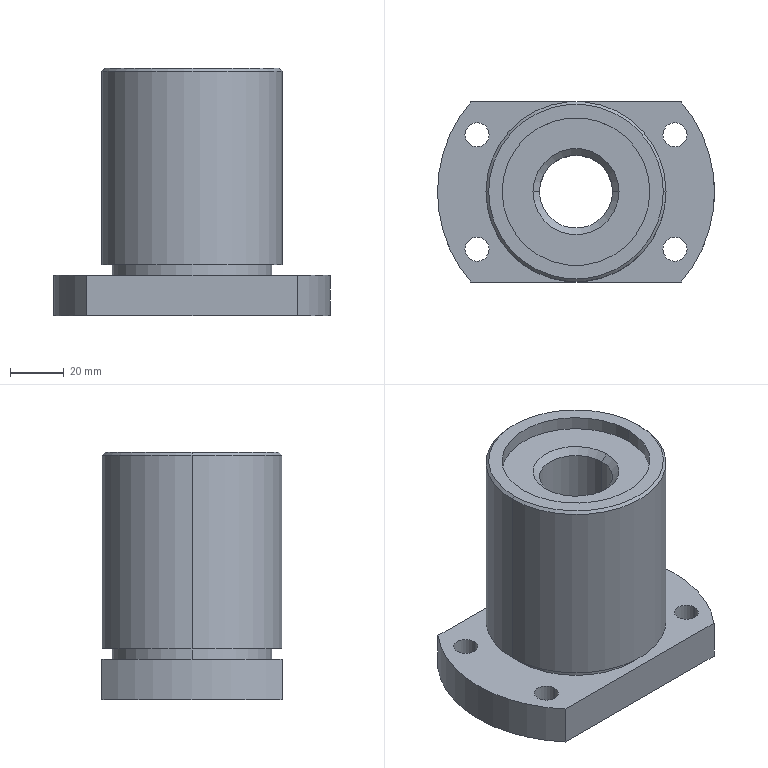Part | SolidWorks | features BaseBody 1 | 1 solid | 39 faces | box 103 x 67 x 92 mm | volume 287626 mm3 | cylinder 23 | cone 8 | plane 8 | commonest cylinder face diameters 9 x8 55 x4 103 x3 4.917 x2 27.2 x2 59.3 x2
STEP:
#1=CARTESIAN_POINT('',(211.71,1592.079,-1039.15));
#2=VERTEX_POINT('',#1);
#3=CARTESIAN_POINT('',(144.71,1592.079,-1039.15));
#4=VERTEX_POINT('',#3);
#5=CARTESIAN_POINT('',(178.21,1592.079,-1039.15));
#6=DIRECTION('',(0.,0.,1.));
#7=DIRECTION('',(1.,0.,0.));
#8=AXIS2_PLACEMENT_3D('',#5,#6,#7);
#9=CIRCLE('',#8,33.5);
#10=EDGE_CURVE('',#2,#4,#9,.T.);
#11=ORIENTED_EDGE('',*,*,#10,.T.);
#12=CARTESIAN_POINT('',(144.71,1592.079,-967.));
#13=VERTEX_POINT('',#12);
#14=CARTESIAN_POINT('',(144.71,1592.079,-1043.));
#15=DIRECTION('',(0.,0.,1.));
#16=VECTOR('',#15,1000.);
#17=LINE('',#14,#16);
#18=EDGE_CURVE('',#4,#13,#17,.T.);
#19=ORIENTED_EDGE('',*,*,#18,.T.);
#20=CARTESIAN_POINT('',(211.71,1592.079,-967.));
#21=VERTEX_POINT('',#20);
#22=CARTESIAN_POINT('',(178.21,1592.079,-967.));
#23=DIRECTION('',(0.,0.,-1.));
#24=DIRECTION('',(1.,0.,0.));
#25=AXIS2_PLACEMENT_3D('',#22,#23,#24);
#26=CIRCLE('',#25,33.5);
#27=EDGE_CURVE('',#13,#21,#26,.T.);
#28=ORIENTED_EDGE('',*,*,#27,.T.);
#29=CARTESIAN_POINT('',(211.71,1592.079,-1043.));
#30=DIRECTION('',(0.,0.,1.));
#31=VECTOR('',#30,1000.);
#32=LINE('',#29,#31);
#33=EDGE_CURVE('',#2,#21,#32,.T.);
#34=ORIENTED_EDGE('',*,*,#33,.F.);
#35=EDGE_LOOP('',(#11,#19,#28,#34));
#36=FACE_OUTER_BOUND('',#35,.T.);
#37=CARTESIAN_POINT('',(178.21,1592.079,-1043.));
#38=DIRECTION('',(0.,0.,1.));
#39=DIRECTION('',(1.,0.,0.));
#40=AXIS2_PLACEMENT_3D('',#37,#38,#39);
#41=CYLINDRICAL_SURFACE('',#40,33.5);
#42=ADVANCED_FACE('',(#36),#41,.T.);
#43=CARTESIAN_POINT('',(145.71,1592.079,-966.));
#44=VERTEX_POINT('',#43);
#45=CARTESIAN_POINT('',(210.71,1592.079,-966.));
#46=VERTEX_POINT('',#45);
#47=CARTESIAN_POINT('',(178.21,1592.079,-966.));
#48=DIRECTION('',(0.,0.,-1.));
#49=DIRECTION('',(-1.,0.,0.));
#50=AXIS2_PLACEMENT_3D('',#47,#48,#49);
#51=CIRCLE('',#50,32.5);
#52=EDGE_CURVE('',#44,#46,#51,.T.);
#53=ORIENTED_EDGE('',*,*,#52,.T.);
#54=CARTESIAN_POINT('',(211.71,1592.079,-967.));
#55=DIRECTION('',(0.7071,0.,-0.7071));
#56=VECTOR('',#55,1000.);
#57=LINE('',#54,#56);
#58=EDGE_CURVE('',#46,#21,#57,.T.);
#59=ORIENTED_EDGE('',*,*,#58,.T.);
#60=ORIENTED_EDGE('',*,*,#27,.F.);
#61=CARTESIAN_POINT('',(144.71,1592.079,-967.));
#62=DIRECTION('',(-0.7071,0.,-0.7071));
#63=VECTOR('',#62,1000.);
#64=LINE('',#61,#63);
#65=EDGE_CURVE('',#44,#13,#64,.T.);
#66=ORIENTED_EDGE('',*,*,#65,.F.);
#67=EDGE_LOOP('',(#53,#59,#60,#66));
#68=FACE_OUTER_BOUND('',#67,.T.);
#69=CARTESIAN_POINT('',(178.21,1592.079,-967.));
#70=DIRECTION('',(0.,0.,-1.));
#71=DIRECTION('',(-1.,0.,0.));
#72=AXIS2_PLACEMENT_3D('',#69,#70,#71);
#73=CONICAL_SURFACE('',#72,33.5,0.7854);
#74=ADVANCED_FACE('',(#68),#73,.T.);
#75=CARTESIAN_POINT('',(207.86,1592.079,-1043.));
#76=VERTEX_POINT('',#75);
#77=CARTESIAN_POINT('',(148.56,1592.079,-1043.));
#78=VERTEX_POINT('',#77);
#79=CARTESIAN_POINT('',(178.21,1592.079,-1043.));
#80=DIRECTION('',(0.,0.,1.));
#81=DIRECTION('',(1.,0.,0.));
#82=AXIS2_PLACEMENT_3D('',#79,#80,#81);
#83=CIRCLE('',#82,29.65);
#84=EDGE_CURVE('',#76,#78,#83,.T.);
#85=ORIENTED_EDGE('',*,*,#84,.T.);
#86=CARTESIAN_POINT('',(148.56,1592.079,-1039.15));
#87=VERTEX_POINT('',#86);
#88=CARTESIAN_POINT('',(148.56,1592.079,-1043.));
#89=DIRECTION('',(0.,0.,1.));
#90=VECTOR('',#89,1000.);
#91=LINE('',#88,#90);
#92=EDGE_CURVE('',#78,#87,#91,.T.);
#93=ORIENTED_EDGE('',*,*,#92,.T.);
#94=CARTESIAN_POINT('',(207.86,1592.079,-1039.15));
#95=VERTEX_POINT('',#94);
#96=CARTESIAN_POINT('',(178.21,1592.079,-1039.15));
#97=DIRECTION('',(0.,0.,-1.));
#98=DIRECTION('',(1.,0.,0.));
#99=AXIS2_PLACEMENT_3D('',#96,#97,#98);
#100=CIRCLE('',#99,29.65);
#101=EDGE_CURVE('',#87,#95,#100,.T.);
#102=ORIENTED_EDGE('',*,*,#101,.T.);
#103=CARTESIAN_POINT('',(207.86,1592.079,-1043.));
#104=DIRECTION('',(0.,0.,1.));
#105=VECTOR('',#104,1000.);
#106=LINE('',#103,#105);
#107=EDGE_CURVE('',#76,#95,#106,.T.);
#108=ORIENTED_EDGE('',*,*,#107,.F.);
#109=EDGE_LOOP('',(#85,#93,#102,#108));
#110=FACE_OUTER_BOUND('',#109,.T.);
#111=CARTESIAN_POINT('',(178.21,1592.079,-1043.));
#112=DIRECTION('',(0.,0.,1.));
#113=DIRECTION('',(1.,0.,0.));
#114=AXIS2_PLACEMENT_3D('',#111,#112,#113);
#115=CYLINDRICAL_SURFACE('',#114,29.65);
#116=ADVANCED_FACE('',(#110),#115,.T.);
#117=CARTESIAN_POINT('',(150.71,1592.079,-971.));
#118=VERTEX_POINT('',#117);
#119=CARTESIAN_POINT('',(205.71,1592.079,-971.));
#120=VERTEX_POINT('',#119);
#121=CARTESIAN_POINT('',(178.21,1592.079,-971.));
#122=DIRECTION('',(0.,0.,1.));
#123=DIRECTION('',(1.,0.,0.));
#124=AXIS2_PLACEMENT_3D('',#121,#122,#123);
#125=CIRCLE('',#124,27.5);
#126=EDGE_CURVE('',#118,#120,#125,.T.);
#127=ORIENTED_EDGE('',*,*,#126,.F.);
#128=CARTESIAN_POINT('',(150.71,1592.079,-966.));
#129=VERTEX_POINT('',#128);
#130=CARTESIAN_POINT('',(150.71,1592.079,-1043.));
#131=DIRECTION('',(0.,0.,1.));
#132=VECTOR('',#131,1000.);
#133=LINE('',#130,#132);
#134=EDGE_CURVE('',#118,#129,#133,.T.);
#135=ORIENTED_EDGE('',*,*,#134,.T.);
#136=CARTESIAN_POINT('',(205.71,1592.079,-966.));
#137=VERTEX_POINT('',#136);
#138=CARTESIAN_POINT('',(178.21,1592.079,-966.));
#139=DIRECTION('',(0.,0.,1.));
#140=DIRECTION('',(1.,0.,0.));
#141=AXIS2_PLACEMENT_3D('',#138,#139,#140);
#142=CIRCLE('',#141,27.5);
#143=EDGE_CURVE('',#129,#137,#142,.T.);
#144=ORIENTED_EDGE('',*,*,#143,.T.);
#145=CARTESIAN_POINT('',(205.71,1592.079,-1043.));
#146=DIRECTION('',(0.,0.,1.));
#147=VECTOR('',#146,1000.);
#148=LINE('',#145,#147);
#149=EDGE_CURVE('',#120,#137,#148,.T.);
#150=ORIENTED_EDGE('',*,*,#149,.F.);
#151=EDGE_LOOP('',(#127,#135,#144,#150));
#152=FACE_OUTER_BOUND('',#151,.T.);
#153=CARTESIAN_POINT('',(178.21,1592.079,-1043.));
#154=DIRECTION('',(0.,0.,1.));
#155=DIRECTION('',(1.,0.,0.));
#156=AXIS2_PLACEMENT_3D('',#153,#154,#155);
#157=CYLINDRICAL_SURFACE('',#156,27.5);
#158=ADVANCED_FACE('',(#152),#157,.F.);
#159=CARTESIAN_POINT('',(136.904,1613.329,-1058.));
#160=VERTEX_POINT('',#159);
#161=CARTESIAN_POINT('',(145.904,1613.329,-1058.));
#162=VERTEX_POINT('',#161);
#163=CARTESIAN_POINT('',(141.404,1613.329,-1058.));
#164=DIRECTION('',(0.,0.,1.));
#165=DIRECTION('',(1.,0.,0.));
#166=AXIS2_PLACEMENT_3D('',#163,#164,#165);
#167=CIRCLE('',#166,4.5);
#168=EDGE_CURVE('',#160,#162,#167,.T.);
#169=ORIENTED_EDGE('',*,*,#168,.F.);
#170=CARTESIAN_POINT('',(136.904,1613.329,-1043.));
#171=VERTEX_POINT('',#170);
#172=CARTESIAN_POINT('',(136.904,1613.329,-1058.));
#173=DIRECTION('',(0.,0.,1.));
#174=VECTOR('',#173,1000.);
#175=LINE('',#172,#174);
#176=EDGE_CURVE('',#160,#171,#175,.T.);
#177=ORIENTED_EDGE('',*,*,#176,.T.);
#178=CARTESIAN_POINT('',(145.904,1613.329,-1043.));
#179=VERTEX_POINT('',#178);
#180=CARTESIAN_POINT('',(141.404,1613.329,-1043.));
#181=DIRECTION('',(0.,0.,1.));
#182=DIRECTION('',(1.,0.,0.));
#183=AXIS2_PLACEMENT_3D('',#180,#181,#182);
#184=CIRCLE('',#183,4.5);
#185=EDGE_CURVE('',#171,#179,#184,.T.);
#186=ORIENTED_EDGE('',*,*,#185,.T.);
#187=CARTESIAN_POINT('',(145.904,1613.329,-1058.));
#188=DIRECTION('',(0.,0.,1.));
#189=VECTOR('',#188,1000.);
#190=LINE('',#187,#189);
#191=EDGE_CURVE('',#162,#179,#190,.T.);
#192=ORIENTED_EDGE('',*,*,#191,.F.);
#193=EDGE_LOOP('',(#169,#177,#186,#192));
#194=FACE_OUTER_BOUND('',#193,.T.);
#195=CARTESIAN_POINT('',(141.404,1613.329,-1058.));
#196=DIRECTION('',(0.,0.,1.));
#197=DIRECTION('',(1.,0.,0.));
#198=AXIS2_PLACEMENT_3D('',#195,#196,#197);
#199=CYLINDRICAL_SURFACE('',#198,4.5);
#200=ADVANCED_FACE('',(#194),#199,.F.);
#201=CARTESIAN_POINT('',(210.516,1570.829,-1058.));
#202=VERTEX_POINT('',#201);
#203=CARTESIAN_POINT('',(219.516,1570.829,-1058.));
#204=VERTEX_POINT('',#203);
#205=CARTESIAN_POINT('',(215.016,1570.829,-1058.));
#206=DIRECTION('',(0.,0.,1.));
#207=DIRECTION('',(1.,0.,0.));
#208=AXIS2_PLACEMENT_3D('',#205,#206,#207);
#209=CIRCLE('',#208,4.5);
#210=EDGE_CURVE('',#202,#204,#209,.T.);
#211=ORIENTED_EDGE('',*,*,#210,.F.);
#212=CARTESIAN_POINT('',(210.516,1570.829,-1043.));
#213=VERTEX_POINT('',#212);
#214=CARTESIAN_POINT('',(210.516,1570.829,-1058.));
#215=DIRECTION('',(0.,0.,1.));
#216=VECTOR('',#215,1000.);
#217=LINE('',#214,#216);
#218=EDGE_CURVE('',#202,#213,#217,.T.);
#219=ORIENTED_EDGE('',*,*,#218,.T.);
#220=CARTESIAN_POINT('',(219.516,1570.829,-1043.));
#221=VERTEX_POINT('',#220);
#222=CARTESIAN_POINT('',(215.016,1570.829,-1043.));
#223=DIRECTION('',(0.,0.,1.));
#224=DIRECTION('',(1.,0.,0.));
#225=AXIS2_PLACEMENT_3D('',#222,#223,#224);
#226=CIRCLE('',#225,4.5);
#227=EDGE_CURVE('',#213,#221,#226,.T.);
#228=ORIENTED_EDGE('',*,*,#227,.T.);
#229=CARTESIAN_POINT('',(219.516,1570.829,-1058.));
#230=DIRECTION('',(0.,0.,1.));
#231=VECTOR('',#230,1000.);
#232=LINE('',#229,#231);
#233=EDGE_CURVE('',#204,#221,#232,.T.);
#234=ORIENTED_EDGE('',*,*,#233,.F.);
#235=EDGE_LOOP('',(#211,#219,#228,#234));
#236=FACE_OUTER_BOUND('',#235,.T.);
#237=CARTESIAN_POINT('',(215.016,1570.829,-1058.));
#238=DIRECTION('',(0.,0.,1.));
#239=DIRECTION('',(1.,0.,0.));
#240=AXIS2_PLACEMENT_3D('',#237,#238,#239);
#241=CYLINDRICAL_SURFACE('',#240,4.5);
#242=ADVANCED_FACE('',(#236),#241,.F.);
#243=CARTESIAN_POINT('',(210.516,1613.329,-1058.));
#244=VERTEX_POINT('',#243);
#245=CARTESIAN_POINT('',(219.516,1613.329,-1058.));
#246=VERTEX_POINT('',#245);
#247=CARTESIAN_POINT('',(215.016,1613.329,-1058.));
#248=DIRECTION('',(0.,0.,1.));
#249=DIRECTION('',(1.,0.,0.));
#250=AXIS2_PLACEMENT_3D('',#247,#248,#249);
#251=CIRCLE('',#250,4.5);
#252=EDGE_CURVE('',#244,#246,#251,.T.);
#253=ORIENTED_EDGE('',*,*,#252,.F.);
#254=CARTESIAN_POINT('',(210.516,1613.329,-1043.));
#255=VERTEX_POINT('',#254);
#256=CARTESIAN_POINT('',(210.516,1613.329,-1058.));
#257=DIRECTION('',(0.,0.,1.));
#258=VECTOR('',#257,1000.);
#259=LINE('',#256,#258);
#260=EDGE_CURVE('',#244,#255,#259,.T.);
#261=ORIENTED_EDGE('',*,*,#260,.T.);
#262=CARTESIAN_POINT('',(219.516,1613.329,-1043.));
#263=VERTEX_POINT('',#262);
#264=CARTESIAN_POINT('',(215.016,1613.329,-1043.));
#265=DIRECTION('',(0.,0.,1.));
#266=DIRECTION('',(1.,0.,0.));
#267=AXIS2_PLACEMENT_3D('',#264,#265,#266);
#268=CIRCLE('',#267,4.5);
#269=EDGE_CURVE('',#255,#263,#268,.T.);
#270=ORIENTED_EDGE('',*,*,#269,.T.);
#271=CARTESIAN_POINT('',(219.516,1613.329,-1058.));
#272=DIRECTION('',(0.,0.,1.));
#273=VECTOR('',#272,1000.);
#274=LINE('',#271,#273);
#275=EDGE_CURVE('',#246,#263,#274,.T.);
#276=ORIENTED_EDGE('',*,*,#275,.F.);
#277=EDGE_LOOP('',(#253,#261,#270,#276));
#278=FACE_OUTER_BOUND('',#277,.T.);
#279=CARTESIAN_POINT('',(215.016,1613.329,-1058.));
#280=DIRECTION('',(0.,0.,1.));
#281=DIRECTION('',(1.,0.,0.));
#282=AXIS2_PLACEMENT_3D('',#279,#280,#281);
#283=CYLINDRICAL_SURFACE('',#282,4.5);
#284=ADVANCED_FACE('',(#278),#283,.F.);
#285=CARTESIAN_POINT('',(136.904,1570.829,-1058.));
#286=VERTEX_POINT('',#285);
#287=CARTESIAN_POINT('',(145.904,1570.829,-1058.));
#288=VERTEX_POINT('',#287);
#289=CARTESIAN_POINT('',(141.404,1570.829,-1058.));
#290=DIRECTION('',(0.,0.,1.));
#291=DIRECTION('',(1.,0.,0.));
#292=AXIS2_PLACEMENT_3D('',#289,#290,#291);
#293=CIRCLE('',#292,4.5);
#294=EDGE_CURVE('',#286,#288,#293,.T.);
#295=ORIENTED_EDGE('',*,*,#294,.F.);
#296=CARTESIAN_POINT('',(136.904,1570.829,-1043.));
#297=VERTEX_POINT('',#296);
#298=CARTESIAN_POINT('',(136.904,1570.829,-1058.));
#299=DIRECTION('',(0.,0.,1.));
#300=VECTOR('',#299,1000.);
#301=LINE('',#298,#300);
#302=EDGE_CURVE('',#286,#297,#301,.T.);
#303=ORIENTED_EDGE('',*,*,#302,.T.);
#304=CARTESIAN_POINT('',(145.904,1570.829,-1043.));
#305=VERTEX_POINT('',#304);
#306=CARTESIAN_POINT('',(141.404,1570.829,-1043.));
#307=DIRECTION('',(0.,0.,1.));
#308=DIRECTION('',(1.,0.,0.));
#309=AXIS2_PLACEMENT_3D('',#306,#307,#308);
#310=CIRCLE('',#309,4.5);
#311=EDGE_CURVE('',#297,#305,#310,.T.);
#312=ORIENTED_EDGE('',*,*,#311,.T.);
#313=CARTESIAN_POINT('',(145.904,1570.829,-1058.));
#314=DIRECTION('',(0.,0.,1.));
#315=VECTOR('',#314,1000.);
#316=LINE('',#313,#315);
#317=EDGE_CURVE('',#288,#305,#316,.T.);
#318=ORIENTED_EDGE('',*,*,#317,.F.);
#319=EDGE_LOOP('',(#295,#303,#312,#318));
#320=FACE_OUTER_BOUND('',#319,.T.);
#321=CARTESIAN_POINT('',(141.404,1570.829,-1058.));
#322=DIRECTION('',(0.,0.,1.));
#323=DIRECTION('',(1.,0.,0.));
#324=AXIS2_PLACEMENT_3D('',#321,#322,#323);
#325=CYLINDRICAL_SURFACE('',#324,4.5);
#326=ADVANCED_FACE('',(#320),#325,.F.);
#327=CARTESIAN_POINT('',(217.325,1558.579,-1058.));
#328=VERTEX_POINT('',#327);
#329=CARTESIAN_POINT('',(229.71,1592.079,-1058.));
#330=VERTEX_POINT('',#329);
#331=CARTESIAN_POINT('',(178.21,1592.079,-1058.));
#332=DIRECTION('',(0.,0.,1.));
#333=DIRECTION('',(1.,0.,0.));
#334=AXIS2_PLACEMENT_3D('',#331,#332,#333);
#335=CIRCLE('',#334,51.5);
#336=EDGE_CURVE('',#328,#330,#335,.T.);
#337=ORIENTED_EDGE('',*,*,#336,.T.);
#338=CARTESIAN_POINT('',(229.71,1592.079,-1051.));
#339=VERTEX_POINT('',#338);
#340=CARTESIAN_POINT('',(229.71,1592.079,-1058.));
#341=DIRECTION('',(0.,0.,1.));
#342=VECTOR('',#341,1000.);
#343=LINE('',#340,#342);
#344=EDGE_CURVE('',#330,#339,#343,.T.);
#345=ORIENTED_EDGE('',*,*,#344,.T.);
#346=CARTESIAN_POINT('',(229.627,1589.161,-1048.));
#347=VERTEX_POINT('',#346);
#348=CARTESIAN_POINT('',(229.71,1592.079,-1051.));
#349=CARTESIAN_POINT('',(229.71,1591.885,-1051.));
#350=CARTESIAN_POINT('',(229.709,1591.69,-1050.98));
#351=CARTESIAN_POINT('',(229.705,1591.312,-1050.901));
#352=CARTESIAN_POINT('',(229.702,1591.128,-1050.843));
#353=CARTESIAN_POINT('',(229.694,1590.77,-1050.689));
#354=CARTESIAN_POINT('',(229.689,1590.601,-1050.594));
#355=CARTESIAN_POINT('',(229.679,1590.285,-1050.374));
#356=CARTESIAN_POINT('',(229.674,1590.136,-1050.246));
#357=CARTESIAN_POINT('',(229.663,1589.868,-1049.967));
#358=CARTESIAN_POINT('',(229.657,1589.748,-1049.815));
#359=CARTESIAN_POINT('',(229.648,1589.54,-1049.49));
#360=CARTESIAN_POINT('',(229.643,1589.45,-1049.315));
#361=CARTESIAN_POINT('',(229.632,1589.236,-1048.778));
#362=CARTESIAN_POINT('',(229.627,1589.161,-1048.39));
#363=CARTESIAN_POINT('',(229.627,1589.161,-1048.));
#364=B_SPLINE_CURVE_WITH_KNOTS('',3,(#348,#349,#350,#351,#352,#353,#354,#355,#356,#357,#358,#359,#360,#361,#362,#363),.UNSPECIFIED.,.F.,.F.,(4,2,2,2,2,2,2,4),(0.004645,0.005225,0.005804,0.006384,0.006964,0.007544,0.008124,0.009283),.UNSPECIFIED.);
#365=EDGE_CURVE('',#339,#347,#364,.T.);
#366=ORIENTED_EDGE('',*,*,#365,.T.);
#367=CARTESIAN_POINT('',(229.71,1592.079,-1045.));
#368=VERTEX_POINT('',#367);
#369=CARTESIAN_POINT('',(229.627,1589.161,-1048.));
#370=CARTESIAN_POINT('',(229.627,1589.161,-1047.805));
#371=CARTESIAN_POINT('',(229.628,1589.18,-1047.612));
#372=CARTESIAN_POINT('',(229.633,1589.252,-1047.232));
#373=CARTESIAN_POINT('',(229.636,1589.307,-1047.043));
#374=CARTESIAN_POINT('',(229.643,1589.45,-1046.685));
#375=CARTESIAN_POINT('',(229.648,1589.538,-1046.514));
#376=CARTESIAN_POINT('',(229.657,1589.746,-1046.188));
#377=CARTESIAN_POINT('',(229.663,1589.868,-1046.033));
#378=CARTESIAN_POINT('',(229.674,1590.138,-1045.752));
#379=CARTESIAN_POINT('',(229.679,1590.285,-1045.626));
#380=CARTESIAN_POINT('',(229.689,1590.602,-1045.405));
#381=CARTESIAN_POINT('',(229.694,1590.774,-1045.31));
#382=CARTESIAN_POINT('',(229.702,1591.128,-1045.157));
#383=CARTESIAN_POINT('',(229.705,1591.311,-1045.099));
#384=CARTESIAN_POINT('',(229.709,1591.692,-1045.02));
#385=CARTESIAN_POINT('',(229.71,1591.886,-1045.));
#386=CARTESIAN_POINT('',(229.71,1592.079,-1045.));
#387=B_SPLINE_CURVE_WITH_KNOTS('',3,(#369,#370,#371,#372,#373,#374,#375,#376,#377,#378,#379,#380,#381,#382,#383,#384,#385,#386),.UNSPECIFIED.,.F.,.F.,(4,2,2,2,2,2,2,2,4),(-0.002294,-0.001715,-0.001136,-0.0005568,0.00002246,0.0006017,0.001181,0.00176,0.002339),.UNSPECIFIED.);
#388=EDGE_CURVE('',#347,#368,#387,.T.);
#389=ORIENTED_EDGE('',*,*,#388,.T.);
#390=CARTESIAN_POINT('',(229.71,1592.079,-1043.));
#391=VERTEX_POINT('',#390);
#392=CARTESIAN_POINT('',(229.71,1592.079,-1058.));
#393=DIRECTION('',(0.,0.,1.));
#394=VECTOR('',#393,1000.);
#395=LINE('',#392,#394);
#396=EDGE_CURVE('',#368,#391,#395,.T.);
#397=ORIENTED_EDGE('',*,*,#396,.T.);
#398=CARTESIAN_POINT('',(217.325,1558.579,-1043.));
#399=VERTEX_POINT('',#398);
#400=CARTESIAN_POINT('',(178.21,1592.079,-1043.));
#401=DIRECTION('',(0.,0.,-1.));
#402=DIRECTION('',(1.,0.,0.));
#403=AXIS2_PLACEMENT_3D('',#400,#401,#402);
#404=CIRCLE('',#403,51.5);
#405=EDGE_CURVE('',#391,#399,#404,.T.);
#406=ORIENTED_EDGE('',*,*,#405,.T.);
#407=CARTESIAN_POINT('',(217.325,1558.579,-1058.));
#408=DIRECTION('',(0.,0.,-1.));
#409=VECTOR('',#408,1000.);
#410=LINE('',#407,#409);
#411=EDGE_CURVE('',#399,#328,#410,.T.);
#412=ORIENTED_EDGE('',*,*,#411,.T.);
#413=EDGE_LOOP('',(#337,#345,#366,#389,#397,#406,#412));
#414=FACE_OUTER_BOUND('',#413,.T.);
#415=CARTESIAN_POINT('',(178.21,1592.079,-1058.));
#416=DIRECTION('',(0.,0.,1.));
#417=DIRECTION('',(1.,0.,0.));
#418=AXIS2_PLACEMENT_3D('',#415,#416,#417);
#419=CYLINDRICAL_SURFACE('',#418,51.5);
#420=ADVANCED_FACE('',(#414),#419,.T.);
#421=CARTESIAN_POINT('',(164.61,1592.079,-973.4));
#422=VERTEX_POINT('',#421);
#423=CARTESIAN_POINT('',(191.81,1592.079,-973.4));
#424=VERTEX_POINT('',#423);
#425=CARTESIAN_POINT('',(178.21,1592.079,-973.4));
#426=DIRECTION('',(0.,0.,1.));
#427=DIRECTION('',(0.,1.,0.));
#428=AXIS2_PLACEMENT_3D('',#425,#426,#427);
#429=CIRCLE('',#428,13.6);
#430=EDGE_CURVE('',#422,#424,#429,.T.);
#431=ORIENTED_EDGE('',*,*,#430,.F.);
#432=CARTESIAN_POINT('',(162.21,1592.079,-971.));
#433=VERTEX_POINT('',#432);
#434=CARTESIAN_POINT('',(162.21,1592.079,-971.));
#435=DIRECTION('',(-0.7071,0.,0.7071));
#436=VECTOR('',#435,1000.);
#437=LINE('',#434,#436);
#438=EDGE_CURVE('',#422,#433,#437,.T.);
#439=ORIENTED_EDGE('',*,*,#438,.T.);
#440=CARTESIAN_POINT('',(194.21,1592.079,-971.));
#441=VERTEX_POINT('',#440);
#442=CARTESIAN_POINT('',(178.21,1592.079,-971.));
#443=DIRECTION('',(0.,0.,1.));
#444=DIRECTION('',(1.,0.,0.));
#445=AXIS2_PLACEMENT_3D('',#442,#443,#444);
#446=CIRCLE('',#445,16.);
#447=EDGE_CURVE('',#433,#441,#446,.T.);
#448=ORIENTED_EDGE('',*,*,#447,.T.);
#449=CARTESIAN_POINT('',(194.21,1592.079,-971.));
#450=DIRECTION('',(0.7071,0.,0.7071));
#451=VECTOR('',#450,1000.);
#452=LINE('',#449,#451);
#453=EDGE_CURVE('',#424,#441,#452,.T.);
#454=ORIENTED_EDGE('',*,*,#453,.F.);
#455=EDGE_LOOP('',(#431,#439,#448,#454));
#456=FACE_OUTER_BOUND('',#455,.T.);
#457=CARTESIAN_POINT('',(178.21,1592.079,-971.));
#458=DIRECTION('',(0.,0.,1.));
#459=DIRECTION('',(1.,0.,0.));
#460=AXIS2_PLACEMENT_3D('',#457,#458,#459);
#461=CONICAL_SURFACE('',#460,16.,0.7854);
#462=ADVANCED_FACE('',(#456),#461,.F.);
#463=CARTESIAN_POINT('',(229.169,1592.079,-1045.542));
#464=VERTEX_POINT('',#463);
#465=CARTESIAN_POINT('',(229.169,1592.079,-1050.458));
#466=VERTEX_POINT('',#465);
#467=CARTESIAN_POINT('',(229.169,1592.079,-1048.));
#468=DIRECTION('',(1.,0.,0.));
#469=DIRECTION('',(0.,-1.,0.));
#470=AXIS2_PLACEMENT_3D('',#467,#468,#469);
#471=CIRCLE('',#470,2.458);
#472=EDGE_CURVE('',#464,#466,#471,.T.);
#473=ORIENTED_EDGE('',*,*,#472,.F.);
#474=CARTESIAN_POINT('',(229.715,1592.079,-1044.996));
#475=DIRECTION('',(0.7071,0.,0.7071));
#476=VECTOR('',#475,1000.);
#477=LINE('',#474,#476);
#478=EDGE_CURVE('',#464,#368,#477,.T.);
#479=ORIENTED_EDGE('',*,*,#478,.T.);
#480=ORIENTED_EDGE('',*,*,#388,.F.);
#481=ORIENTED_EDGE('',*,*,#365,.F.);
#482=CARTESIAN_POINT('',(229.715,1592.079,-1051.004));
#483=DIRECTION('',(0.7071,0.,-0.7071));
#484=VECTOR('',#483,1000.);
#485=LINE('',#482,#484);
#486=EDGE_CURVE('',#466,#339,#485,.T.);
#487=ORIENTED_EDGE('',*,*,#486,.F.);
#488=EDGE_LOOP('',(#473,#479,#480,#481,#487));
#489=FACE_OUTER_BOUND('',#488,.T.);
#490=CARTESIAN_POINT('',(229.715,1592.079,-1048.));
#491=DIRECTION('',(1.,0.,0.));
#492=DIRECTION('',(0.,0.,-1.));
#493=AXIS2_PLACEMENT_3D('',#490,#491,#492);
#494=CONICAL_SURFACE('',#493,3.004,0.7854);
#495=ADVANCED_FACE('',(#489),#494,.F.);
#496=CARTESIAN_POINT('',(164.61,1592.079,-1050.6));
#497=VERTEX_POINT('',#496);
#498=CARTESIAN_POINT('',(191.81,1592.079,-1050.6));
#499=VERTEX_POINT('',#498);
#500=CARTESIAN_POINT('',(178.21,1592.079,-1050.6));
#501=DIRECTION('',(0.,0.,1.));
#502=DIRECTION('',(1.,0.,0.));
#503=AXIS2_PLACEMENT_3D('',#500,#501,#502);
#504=CIRCLE('',#503,13.6);
#505=EDGE_CURVE('',#497,#499,#504,.T.);
#506=ORIENTED_EDGE('',*,*,#505,.F.);
#507=CARTESIAN_POINT('',(164.61,1592.079,-1053.));
#508=DIRECTION('',(0.,0.,1.));
#509=VECTOR('',#508,1000.);
#510=LINE('',#507,#509);
#511=EDGE_CURVE('',#497,#422,#510,.T.);
#512=ORIENTED_EDGE('',*,*,#511,.T.);
#513=ORIENTED_EDGE('',*,*,#430,.T.);
#514=CARTESIAN_POINT('',(191.81,1592.079,-1045.542));
#515=VERTEX_POINT('',#514);
#516=CARTESIAN_POINT('',(191.81,1592.079,-1053.));
#517=DIRECTION('',(0.,0.,1.));
#518=VECTOR('',#517,1000.);
#519=LINE('',#516,#518);
#520=EDGE_CURVE('',#515,#424,#519,.T.);
#521=ORIENTED_EDGE('',*,*,#520,.F.);
#522=CARTESIAN_POINT('',(191.81,1592.079,-1050.458));
#523=VERTEX_POINT('',#522);
#524=CARTESIAN_POINT('',(191.81,1592.079,-1050.458));
#525=CARTESIAN_POINT('',(191.81,1591.918,-1050.459));
#526=CARTESIAN_POINT('',(191.807,1591.755,-1050.442));
#527=CARTESIAN_POINT('',(191.796,1591.439,-1050.379));
#528=CARTESIAN_POINT('',(191.788,1591.286,-1050.333));
#529=CARTESIAN_POINT('',(191.767,1590.988,-1050.209));
#530=CARTESIAN_POINT('',(191.755,1590.844,-1050.132));
#531=CARTESIAN_POINT('',(191.728,1590.579,-1049.954));
#532=CARTESIAN_POINT('',(191.713,1590.454,-1049.852));
#533=CARTESIAN_POINT('',(191.684,1590.225,-1049.624));
#534=CARTESIAN_POINT('',(191.669,1590.124,-1049.5));
#535=CARTESIAN_POINT('',(191.642,1589.946,-1049.234));
#536=CARTESIAN_POINT('',(191.63,1589.869,-1049.09));
#537=CARTESIAN_POINT('',(191.609,1589.746,-1048.793));
#538=CARTESIAN_POINT('',(191.6,1589.699,-1048.64));
#539=CARTESIAN_POINT('',(191.589,1589.636,-1048.324));
#540=CARTESIAN_POINT('',(191.586,1589.62,-1048.161));
#541=CARTESIAN_POINT('',(191.586,1589.62,-1047.835));
#542=CARTESIAN_POINT('',(191.589,1589.636,-1047.675));
#543=CARTESIAN_POINT('',(191.6,1589.699,-1047.361));
#544=CARTESIAN_POINT('',(191.609,1589.747,-1047.205));
#545=CARTESIAN_POINT('',(191.63,1589.87,-1046.907));
#546=CARTESIAN_POINT('',(191.642,1589.946,-1046.766));
#547=CARTESIAN_POINT('',(191.669,1590.125,-1046.499));
#548=CARTESIAN_POINT('',(191.684,1590.228,-1046.373));
#549=CARTESIAN_POINT('',(191.728,1590.568,-1046.034));
#550=CARTESIAN_POINT('',(191.757,1590.842,-1045.851));
#551=CARTESIAN_POINT('',(191.788,1591.285,-1045.667));
#552=CARTESIAN_POINT('',(191.796,1591.441,-1045.62));
#553=CARTESIAN_POINT('',(191.807,1591.758,-1045.557));
#554=CARTESIAN_POINT('',(191.81,1591.918,-1045.542));
#555=CARTESIAN_POINT('',(191.81,1592.079,-1045.542));
#556=B_SPLINE_CURVE_WITH_KNOTS('',3,(#524,#525,#526,#527,#528,#529,#530,#531,#532,#533,#534,#535,#536,#537,#538,#539,#540,#541,#542,#543,#544,#545,#546,#547,#548,#549,#550,#551,#552,#553,#554,#555),.UNSPECIFIED.,.F.,.F.,(4,2,2,2,2,2,2,2,2,2,2,2,2,2,2,4),(0.003852,0.004333,0.004815,0.005296,0.005777,0.006258,0.00674,0.007221,0.007702,0.008183,0.008665,0.009146,0.009627,0.01059,0.01107,0.01155),.UNSPECIFIED.);
#557=EDGE_CURVE('',#523,#515,#556,.T.);
#558=ORIENTED_EDGE('',*,*,#557,.F.);
#559=CARTESIAN_POINT('',(191.81,1592.079,-1053.));
#560=DIRECTION('',(0.,0.,1.));
#561=VECTOR('',#560,1000.);
#562=LINE('',#559,#561);
#563=EDGE_CURVE('',#499,#523,#562,.T.);
#564=ORIENTED_EDGE('',*,*,#563,.F.);
#565=EDGE_LOOP('',(#506,#512,#513,#521,#558,#564));
#566=FACE_OUTER_BOUND('',#565,.T.);
#567=CARTESIAN_POINT('',(178.21,1592.079,-1053.));
#568=DIRECTION('',(0.,0.,1.));
#569=DIRECTION('',(1.,0.,0.));
#570=AXIS2_PLACEMENT_3D('',#567,#568,#569);
#571=CYLINDRICAL_SURFACE('',#570,13.6);
#572=ADVANCED_FACE('',(#566),#571,.F.);
#573=CARTESIAN_POINT('',(205.71,1592.079,-1053.));
#574=VERTEX_POINT('',#573);
#575=CARTESIAN_POINT('',(150.71,1592.079,-1053.));
#576=VERTEX_POINT('',#575);
#577=CARTESIAN_POINT('',(178.21,1592.079,-1053.));
#578=DIRECTION('',(0.,0.,-1.));
#579=DIRECTION('',(-1.,0.,0.));
#580=AXIS2_PLACEMENT_3D('',#577,#578,#579);
#581=CIRCLE('',#580,27.5);
#582=EDGE_CURVE('',#574,#576,#581,.T.);
#583=ORIENTED_EDGE('',*,*,#582,.F.);
#584=CARTESIAN_POINT('',(205.71,1592.079,-1058.));
#585=VERTEX_POINT('',#584);
#586=CARTESIAN_POINT('',(205.71,1592.079,-1053.));
#587=DIRECTION('',(0.,0.,-1.));
#588=VECTOR('',#587,1000.);
#589=LINE('',#586,#588);
#590=EDGE_CURVE('',#574,#585,#589,.T.);
#591=ORIENTED_EDGE('',*,*,#590,.T.);
#592=CARTESIAN_POINT('',(150.71,1592.079,-1058.));
#593=VERTEX_POINT('',#592);
#594=CARTESIAN_POINT('',(178.21,1592.079,-1058.));
#595=DIRECTION('',(0.,0.,1.));
#596=DIRECTION('',(-1.,0.,0.));
#597=AXIS2_PLACEMENT_3D('',#594,#595,#596);
#598=CIRCLE('',#597,27.5);
#599=EDGE_CURVE('',#593,#585,#598,.T.);
#600=ORIENTED_EDGE('',*,*,#599,.F.);
#601=CARTESIAN_POINT('',(150.71,1592.079,-1053.));
#602=DIRECTION('',(0.,0.,-1.));
#603=VECTOR('',#602,1000.);
#604=LINE('',#601,#603);
#605=EDGE_CURVE('',#576,#593,#604,.T.);
#606=ORIENTED_EDGE('',*,*,#605,.F.);
#607=EDGE_LOOP('',(#583,#591,#600,#606));
#608=FACE_OUTER_BOUND('',#607,.T.);
#609=CARTESIAN_POINT('',(178.21,1592.079,-1053.));
#610=DIRECTION('',(0.,0.,-1.));
#611=DIRECTION('',(-1.,0.,0.));
#612=AXIS2_PLACEMENT_3D('',#609,#610,#611);
#613=CYLINDRICAL_SURFACE('',#612,27.5);
#614=ADVANCED_FACE('',(#608),#613,.F.);
#615=ORIENTED_EDGE('',*,*,#472,.T.);
#616=CARTESIAN_POINT('',(229.71,1592.079,-1050.458));
#617=DIRECTION('',(-1.,0.,0.));
#618=VECTOR('',#617,1000.);
#619=LINE('',#616,#618);
#620=EDGE_CURVE('',#466,#523,#619,.T.);
#621=ORIENTED_EDGE('',*,*,#620,.T.);
#622=ORIENTED_EDGE('',*,*,#557,.T.);
#623=CARTESIAN_POINT('',(229.71,1592.079,-1045.542));
#624=DIRECTION('',(-1.,0.,0.));
#625=VECTOR('',#624,1000.);
#626=LINE('',#623,#625);
#627=EDGE_CURVE('',#464,#515,#626,.T.);
#628=ORIENTED_EDGE('',*,*,#627,.F.);
#629=EDGE_LOOP('',(#615,#621,#622,#628));
#630=FACE_OUTER_BOUND('',#629,.T.);
#631=CARTESIAN_POINT('',(229.71,1592.079,-1048.));
#632=DIRECTION('',(-1.,0.,0.));
#633=DIRECTION('',(0.,0.,1.));
#634=AXIS2_PLACEMENT_3D('',#631,#632,#633);
#635=CYLINDRICAL_SURFACE('',#634,2.458);
#636=ADVANCED_FACE('',(#630),#635,.F.);
#637=ORIENTED_EDGE('',*,*,#505,.T.);
#638=CARTESIAN_POINT('',(194.21,1592.079,-1053.));
#639=VERTEX_POINT('',#638);
#640=CARTESIAN_POINT('',(194.21,1592.079,-1053.));
#641=DIRECTION('',(0.7071,0.,-0.7071));
#642=VECTOR('',#641,1000.);
#643=LINE('',#640,#642);
#644=EDGE_CURVE('',#499,#639,#643,.T.);
#645=ORIENTED_EDGE('',*,*,#644,.T.);
#646=CARTESIAN_POINT('',(162.21,1592.079,-1053.));
#647=VERTEX_POINT('',#646);
#648=CARTESIAN_POINT('',(178.21,1592.079,-1053.));
#649=DIRECTION('',(0.,0.,1.));
#650=DIRECTION('',(-1.,0.,0.));
#651=AXIS2_PLACEMENT_3D('',#648,#649,#650);
#652=CIRCLE('',#651,16.);
#653=EDGE_CURVE('',#647,#639,#652,.T.);
#654=ORIENTED_EDGE('',*,*,#653,.F.);
#655=CARTESIAN_POINT('',(162.21,1592.079,-1053.));
#656=DIRECTION('',(-0.7071,0.,-0.7071));
#657=VECTOR('',#656,1000.);
#658=LINE('',#655,#657);
#659=EDGE_CURVE('',#497,#647,#658,.T.);
#660=ORIENTED_EDGE('',*,*,#659,.F.);
#661=EDGE_LOOP('',(#637,#645,#654,#660));
#662=FACE_OUTER_BOUND('',#661,.T.);
#663=CARTESIAN_POINT('',(178.21,1592.079,-1053.));
#664=DIRECTION('',(0.,0.,-1.));
#665=DIRECTION('',(-1.,0.,0.));
#666=AXIS2_PLACEMENT_3D('',#663,#664,#665);
#667=CONICAL_SURFACE('',#666,16.,0.7854);
#668=ADVANCED_FACE('',(#662),#667,.F.);
#669=ORIENTED_EDGE('',*,*,#18,.F.);
#670=CARTESIAN_POINT('',(178.21,1592.079,-1039.15));
#671=DIRECTION('',(0.,0.,1.));
#672=DIRECTION('',(1.,0.,0.));
#673=AXIS2_PLACEMENT_3D('',#670,#671,#672);
#674=CIRCLE('',#673,33.5);
#675=EDGE_CURVE('',#4,#2,#674,.T.);
#676=ORIENTED_EDGE('',*,*,#675,.T.);
#677=ORIENTED_EDGE('',*,*,#33,.T.);
#678=CARTESIAN_POINT('',(178.21,1592.079,-967.));
#679=DIRECTION('',(0.,0.,-1.));
#680=DIRECTION('',(1.,0.,0.));
#681=AXIS2_PLACEMENT_3D('',#678,#679,#680);
#682=CIRCLE('',#681,33.5);
#683=EDGE_CURVE('',#21,#13,#682,.T.);
#684=ORIENTED_EDGE('',*,*,#683,.T.);
#685=EDGE_LOOP('',(#669,#676,#677,#684));
#686=FACE_OUTER_BOUND('',#685,.T.);
#687=CARTESIAN_POINT('',(178.21,1592.079,-1043.));
#688=DIRECTION('',(0.,0.,1.));
#689=DIRECTION('',(1.,0.,0.));
#690=AXIS2_PLACEMENT_3D('',#687,#688,#689);
#691=CYLINDRICAL_SURFACE('',#690,33.5);
#692=ADVANCED_FACE('',(#686),#691,.T.);
#693=ORIENTED_EDGE('',*,*,#58,.F.);
#694=CARTESIAN_POINT('',(178.21,1592.079,-966.));
#695=DIRECTION('',(0.,0.,-1.));
#696=DIRECTION('',(-1.,0.,0.));
#697=AXIS2_PLACEMENT_3D('',#694,#695,#696);
#698=CIRCLE('',#697,32.5);
#699=EDGE_CURVE('',#46,#44,#698,.T.);
#700=ORIENTED_EDGE('',*,*,#699,.T.);
#701=ORIENTED_EDGE('',*,*,#65,.T.);
#702=ORIENTED_EDGE('',*,*,#683,.F.);
#703=EDGE_LOOP('',(#693,#700,#701,#702));
#704=FACE_OUTER_BOUND('',#703,.T.);
#705=CARTESIAN_POINT('',(178.21,1592.079,-967.));
#706=DIRECTION('',(0.,0.,-1.));
#707=DIRECTION('',(-1.,0.,0.));
#708=AXIS2_PLACEMENT_3D('',#705,#706,#707);
#709=CONICAL_SURFACE('',#708,33.5,0.7854);
#710=ADVANCED_FACE('',(#704),#709,.T.);
#711=CARTESIAN_POINT('',(178.21,1592.079,-1039.15));
#712=DIRECTION('',(0.,0.,-1.));
#713=DIRECTION('',(1.,0.,0.));
#714=AXIS2_PLACEMENT_3D('',#711,#712,#713);
#715=CIRCLE('',#714,29.65);
#716=EDGE_CURVE('',#95,#87,#715,.T.);
#717=ORIENTED_EDGE('',*,*,#716,.F.);
#718=ORIENTED_EDGE('',*,*,#101,.F.);
#719=EDGE_LOOP('',(#717,#718));
#720=FACE_BOUND('',#719,.T.);
#721=ORIENTED_EDGE('',*,*,#10,.F.);
#722=ORIENTED_EDGE('',*,*,#675,.F.);
#723=EDGE_LOOP('',(#721,#722));
#724=FACE_OUTER_BOUND('',#723,.T.);
#725=CARTESIAN_POINT('',(144.71,1592.079,-1039.15));
#726=DIRECTION('',(0.,0.,1.));
#727=DIRECTION('',(1.,0.,0.));
#728=AXIS2_PLACEMENT_3D('',#725,#726,#727);
#729=PLANE('',#728);
#730=ADVANCED_FACE('',(#720,#724),#729,.F.);
#731=CARTESIAN_POINT('',(178.21,1592.079,-966.));
#732=DIRECTION('',(0.,0.,1.));
#733=DIRECTION('',(1.,0.,0.));
#734=AXIS2_PLACEMENT_3D('',#731,#732,#733);
#735=CIRCLE('',#734,27.5);
#736=EDGE_CURVE('',#137,#129,#735,.T.);
#737=ORIENTED_EDGE('',*,*,#736,.F.);
#738=ORIENTED_EDGE('',*,*,#143,.F.);
#739=EDGE_LOOP('',(#737,#738));
#740=FACE_BOUND('',#739,.T.);
#741=ORIENTED_EDGE('',*,*,#52,.F.);
#742=ORIENTED_EDGE('',*,*,#699,.F.);
#743=EDGE_LOOP('',(#741,#742));
#744=FACE_OUTER_BOUND('',#743,.T.);
#745=CARTESIAN_POINT('',(150.71,1592.079,-966.));
#746=DIRECTION('',(0.,0.,-1.));
#747=DIRECTION('',(-1.,0.,0.));
#748=AXIS2_PLACEMENT_3D('',#745,#746,#747);
#749=PLANE('',#748);
#750=ADVANCED_FACE('',(#740,#744),#749,.F.);
#751=ORIENTED_EDGE('',*,*,#92,.F.);
#752=CARTESIAN_POINT('',(178.21,1592.079,-1043.));
#753=DIRECTION('',(0.,0.,1.));
#754=DIRECTION('',(1.,0.,0.));
#755=AXIS2_PLACEMENT_3D('',#752,#753,#754);
#756=CIRCLE('',#755,29.65);
#757=EDGE_CURVE('',#78,#76,#756,.T.);
#758=ORIENTED_EDGE('',*,*,#757,.T.);
#759=ORIENTED_EDGE('',*,*,#107,.T.);
#760=ORIENTED_EDGE('',*,*,#716,.T.);
#761=EDGE_LOOP('',(#751,#758,#759,#760));
#762=FACE_OUTER_BOUND('',#761,.T.);
#763=CARTESIAN_POINT('',(178.21,1592.079,-1043.));
#764=DIRECTION('',(0.,0.,1.));
#765=DIRECTION('',(1.,0.,0.));
#766=AXIS2_PLACEMENT_3D('',#763,#764,#765);
#767=CYLINDRICAL_SURFACE('',#766,29.65);
#768=ADVANCED_FACE('',(#762),#767,.T.);
#769=ORIENTED_EDGE('',*,*,#134,.F.);
#770=CARTESIAN_POINT('',(178.21,1592.079,-971.));
#771=DIRECTION('',(0.,0.,1.));
#772=DIRECTION('',(1.,0.,0.));
#773=AXIS2_PLACEMENT_3D('',#770,#771,#772);
#774=CIRCLE('',#773,27.5);
#775=EDGE_CURVE('',#120,#118,#774,.T.);
#776=ORIENTED_EDGE('',*,*,#775,.F.);
#777=ORIENTED_EDGE('',*,*,#149,.T.);
#778=ORIENTED_EDGE('',*,*,#736,.T.);
#779=EDGE_LOOP('',(#769,#776,#777,#778));
#780=FACE_OUTER_BOUND('',#779,.T.);
#781=CARTESIAN_POINT('',(178.21,1592.079,-1043.));
#782=DIRECTION('',(0.,0.,1.));
#783=DIRECTION('',(1.,0.,0.));
#784=AXIS2_PLACEMENT_3D('',#781,#782,#783);
#785=CYLINDRICAL_SURFACE('',#784,27.5);
#786=ADVANCED_FACE('',(#780),#785,.F.);
#787=ORIENTED_EDGE('',*,*,#84,.F.);
#788=ORIENTED_EDGE('',*,*,#757,.F.);
#789=EDGE_LOOP('',(#787,#788));
#790=FACE_BOUND('',#789,.T.);
#791=CARTESIAN_POINT('',(141.404,1613.329,-1043.));
#792=DIRECTION('',(0.,0.,1.));
#793=DIRECTION('',(1.,0.,0.));
#794=AXIS2_PLACEMENT_3D('',#791,#792,#793);
#795=CIRCLE('',#794,4.5);
#796=EDGE_CURVE('',#179,#171,#795,.T.);
#797=ORIENTED_EDGE('',*,*,#796,.F.);
#798=ORIENTED_EDGE('',*,*,#185,.F.);
#799=EDGE_LOOP('',(#797,#798));
#800=FACE_BOUND('',#799,.T.);
#801=CARTESIAN_POINT('',(215.016,1570.829,-1043.));
#802=DIRECTION('',(0.,0.,1.));
#803=DIRECTION('',(1.,0.,0.));
#804=AXIS2_PLACEMENT_3D('',#801,#802,#803);
#805=CIRCLE('',#804,4.5);
#806=EDGE_CURVE('',#221,#213,#805,.T.);
#807=ORIENTED_EDGE('',*,*,#806,.F.);
#808=ORIENTED_EDGE('',*,*,#227,.F.);
#809=EDGE_LOOP('',(#807,#808));
#810=FACE_BOUND('',#809,.T.);
#811=CARTESIAN_POINT('',(215.016,1613.329,-1043.));
#812=DIRECTION('',(0.,0.,1.));
#813=DIRECTION('',(1.,0.,0.));
#814=AXIS2_PLACEMENT_3D('',#811,#812,#813);
#815=CIRCLE('',#814,4.5);
#816=EDGE_CURVE('',#263,#255,#815,.T.);
#817=ORIENTED_EDGE('',*,*,#816,.F.);
#818=ORIENTED_EDGE('',*,*,#269,.F.);
#819=EDGE_LOOP('',(#817,#818));
#820=FACE_BOUND('',#819,.T.);
#821=CARTESIAN_POINT('',(141.404,1570.829,-1043.));
#822=DIRECTION('',(0.,0.,1.));
#823=DIRECTION('',(1.,0.,0.));
#824=AXIS2_PLACEMENT_3D('',#821,#822,#823);
#825=CIRCLE('',#824,4.5);
#826=EDGE_CURVE('',#305,#297,#825,.T.);
#827=ORIENTED_EDGE('',*,*,#826,.F.);
#828=ORIENTED_EDGE('',*,*,#311,.F.);
#829=EDGE_LOOP('',(#827,#828));
#830=FACE_BOUND('',#829,.T.);
#831=CARTESIAN_POINT('',(217.325,1625.579,-1043.));
#832=VERTEX_POINT('',#831);
#833=CARTESIAN_POINT('',(178.21,1592.079,-1043.));
#834=DIRECTION('',(0.,0.,-1.));
#835=DIRECTION('',(1.,0.,0.));
#836=AXIS2_PLACEMENT_3D('',#833,#834,#835);
#837=CIRCLE('',#836,51.5);
#838=EDGE_CURVE('',#832,#391,#837,.T.);
#839=ORIENTED_EDGE('',*,*,#838,.F.);
#840=CARTESIAN_POINT('',(139.095,1625.579,-1043.));
#841=VERTEX_POINT('',#840);
#842=CARTESIAN_POINT('',(178.21,1625.579,-1043.));
#843=DIRECTION('',(1.,0.,0.));
#844=VECTOR('',#843,1000.);
#845=LINE('',#842,#844);
#846=EDGE_CURVE('',#841,#832,#845,.T.);
#847=ORIENTED_EDGE('',*,*,#846,.F.);
#848=CARTESIAN_POINT('',(139.095,1558.579,-1043.));
#849=VERTEX_POINT('',#848);
#850=CARTESIAN_POINT('',(178.21,1592.079,-1043.));
#851=DIRECTION('',(0.,0.,-1.));
#852=DIRECTION('',(1.,0.,0.));
#853=AXIS2_PLACEMENT_3D('',#850,#851,#852);
#854=CIRCLE('',#853,51.5);
#855=EDGE_CURVE('',#849,#841,#854,.T.);
#856=ORIENTED_EDGE('',*,*,#855,.F.);
#857=CARTESIAN_POINT('',(178.21,1558.579,-1043.));
#858=DIRECTION('',(-1.,0.,0.));
#859=VECTOR('',#858,1000.);
#860=LINE('',#857,#859);
#861=EDGE_CURVE('',#399,#849,#860,.T.);
#862=ORIENTED_EDGE('',*,*,#861,.F.);
#863=ORIENTED_EDGE('',*,*,#405,.F.);
#864=EDGE_LOOP('',(#839,#847,#856,#862,#863));
#865=FACE_OUTER_BOUND('',#864,.T.);
#866=CARTESIAN_POINT('',(178.21,1592.079,-1043.));
#867=DIRECTION('',(0.,0.,-1.));
#868=DIRECTION('',(-1.,0.,0.));
#869=AXIS2_PLACEMENT_3D('',#866,#867,#868);
#870=PLANE('',#869);
#871=ADVANCED_FACE('',(#790,#800,#810,#820,#830,#865),#870,.F.);
#872=CARTESIAN_POINT('',(178.21,1592.079,-971.));
#873=DIRECTION('',(0.,0.,1.));
#874=DIRECTION('',(1.,0.,0.));
#875=AXIS2_PLACEMENT_3D('',#872,#873,#874);
#876=CIRCLE('',#875,16.);
#877=EDGE_CURVE('',#441,#433,#876,.T.);
#878=ORIENTED_EDGE('',*,*,#877,.F.);
#879=ORIENTED_EDGE('',*,*,#447,.F.);
#880=EDGE_LOOP('',(#878,#879));
#881=FACE_BOUND('',#880,.T.);
#882=ORIENTED_EDGE('',*,*,#775,.T.);
#883=ORIENTED_EDGE('',*,*,#126,.T.);
#884=EDGE_LOOP('',(#882,#883));
#885=FACE_OUTER_BOUND('',#884,.T.);
#886=CARTESIAN_POINT('',(178.21,1592.079,-971.));
#887=DIRECTION('',(0.,0.,-1.));
#888=DIRECTION('',(-1.,0.,0.));
#889=AXIS2_PLACEMENT_3D('',#886,#887,#888);
#890=PLANE('',#889);
#891=ADVANCED_FACE('',(#881,#885),#890,.F.);
#892=ORIENTED_EDGE('',*,*,#176,.F.);
#893=CARTESIAN_POINT('',(141.404,1613.329,-1058.));
#894=DIRECTION('',(0.,0.,1.));
#895=DIRECTION('',(1.,0.,0.));
#896=AXIS2_PLACEMENT_3D('',#893,#894,#895);
#897=CIRCLE('',#896,4.5);
#898=EDGE_CURVE('',#162,#160,#897,.T.);
#899=ORIENTED_EDGE('',*,*,#898,.F.);
#900=ORIENTED_EDGE('',*,*,#191,.T.);
#901=ORIENTED_EDGE('',*,*,#796,.T.);
#902=EDGE_LOOP('',(#892,#899,#900,#901));
#903=FACE_OUTER_BOUND('',#902,.T.);
#904=CARTESIAN_POINT('',(141.404,1613.329,-1058.));
#905=DIRECTION('',(0.,0.,1.));
#906=DIRECTION('',(1.,0.,0.));
#907=AXIS2_PLACEMENT_3D('',#904,#905,#906);
#908=CYLINDRICAL_SURFACE('',#907,4.5);
#909=ADVANCED_FACE('',(#903),#908,.F.);
#910=ORIENTED_EDGE('',*,*,#218,.F.);
#911=CARTESIAN_POINT('',(215.016,1570.829,-1058.));
#912=DIRECTION('',(0.,0.,1.));
#913=DIRECTION('',(1.,0.,0.));
#914=AXIS2_PLACEMENT_3D('',#911,#912,#913);
#915=CIRCLE('',#914,4.5);
#916=EDGE_CURVE('',#204,#202,#915,.T.);
#917=ORIENTED_EDGE('',*,*,#916,.F.);
#918=ORIENTED_EDGE('',*,*,#233,.T.);
#919=ORIENTED_EDGE('',*,*,#806,.T.);
#920=EDGE_LOOP('',(#910,#917,#918,#919));
#921=FACE_OUTER_BOUND('',#920,.T.);
#922=CARTESIAN_POINT('',(215.016,1570.829,-1058.));
#923=DIRECTION('',(0.,0.,1.));
#924=DIRECTION('',(1.,0.,0.));
#925=AXIS2_PLACEMENT_3D('',#922,#923,#924);
#926=CYLINDRICAL_SURFACE('',#925,4.5);
#927=ADVANCED_FACE('',(#921),#926,.F.);
#928=ORIENTED_EDGE('',*,*,#260,.F.);
#929=CARTESIAN_POINT('',(215.016,1613.329,-1058.));
#930=DIRECTION('',(0.,0.,1.));
#931=DIRECTION('',(1.,0.,0.));
#932=AXIS2_PLACEMENT_3D('',#929,#930,#931);
#933=CIRCLE('',#932,4.5);
#934=EDGE_CURVE('',#246,#244,#933,.T.);
#935=ORIENTED_EDGE('',*,*,#934,.F.);
#936=ORIENTED_EDGE('',*,*,#275,.T.);
#937=ORIENTED_EDGE('',*,*,#816,.T.);
#938=EDGE_LOOP('',(#928,#935,#936,#937));
#939=FACE_OUTER_BOUND('',#938,.T.);
#940=CARTESIAN_POINT('',(215.016,1613.329,-1058.));
#941=DIRECTION('',(0.,0.,1.));
#942=DIRECTION('',(1.,0.,0.));
#943=AXIS2_PLACEMENT_3D('',#940,#941,#942);
#944=CYLINDRICAL_SURFACE('',#943,4.5);
#945=ADVANCED_FACE('',(#939),#944,.F.);
#946=ORIENTED_EDGE('',*,*,#302,.F.);
#947=CARTESIAN_POINT('',(141.404,1570.829,-1058.));
#948=DIRECTION('',(0.,0.,1.));
#949=DIRECTION('',(1.,0.,0.));
#950=AXIS2_PLACEMENT_3D('',#947,#948,#949);
#951=CIRCLE('',#950,4.5);
#952=EDGE_CURVE('',#288,#286,#951,.T.);
#953=ORIENTED_EDGE('',*,*,#952,.F.);
#954=ORIENTED_EDGE('',*,*,#317,.T.);
#955=ORIENTED_EDGE('',*,*,#826,.T.);
#956=EDGE_LOOP('',(#946,#953,#954,#955));
#957=FACE_OUTER_BOUND('',#956,.T.);
#958=CARTESIAN_POINT('',(141.404,1570.829,-1058.));
#959=DIRECTION('',(0.,0.,1.));
#960=DIRECTION('',(1.,0.,0.));
#961=AXIS2_PLACEMENT_3D('',#958,#959,#960);
#962=CYLINDRICAL_SURFACE('',#961,4.5);
#963=ADVANCED_FACE('',(#957),#962,.F.);
#964=CARTESIAN_POINT('',(139.095,1558.579,-1058.));
#965=VERTEX_POINT('',#964);
#966=CARTESIAN_POINT('',(217.325,1558.579,-1058.));
#967=DIRECTION('',(-1.,0.,0.));
#968=VECTOR('',#967,1000.);
#969=LINE('',#966,#968);
#970=EDGE_CURVE('',#328,#965,#969,.T.);
#971=ORIENTED_EDGE('',*,*,#970,.F.);
#972=ORIENTED_EDGE('',*,*,#411,.F.);
#973=ORIENTED_EDGE('',*,*,#861,.T.);
#974=CARTESIAN_POINT('',(139.095,1558.579,-1058.));
#975=DIRECTION('',(0.,0.,1.));
#976=VECTOR('',#975,1000.);
#977=LINE('',#974,#976);
#978=EDGE_CURVE('',#965,#849,#977,.T.);
#979=ORIENTED_EDGE('',*,*,#978,.F.);
#980=EDGE_LOOP('',(#971,#972,#973,#979));
#981=FACE_OUTER_BOUND('',#980,.T.);
#982=CARTESIAN_POINT('',(217.325,1558.579,-1058.));
#983=DIRECTION('',(0.,1.,0.));
#984=DIRECTION('',(0.,0.,1.));
#985=AXIS2_PLACEMENT_3D('',#982,#983,#984);
#986=PLANE('',#985);
#987=ADVANCED_FACE('',(#981),#986,.F.);
#988=ORIENTED_EDGE('',*,*,#344,.F.);
#989=CARTESIAN_POINT('',(217.325,1625.579,-1058.));
#990=VERTEX_POINT('',#989);
#991=CARTESIAN_POINT('',(178.21,1592.079,-1058.));
#992=DIRECTION('',(0.,0.,1.));
#993=DIRECTION('',(1.,0.,0.));
#994=AXIS2_PLACEMENT_3D('',#991,#992,#993);
#995=CIRCLE('',#994,51.5);
#996=EDGE_CURVE('',#330,#990,#995,.T.);
#997=ORIENTED_EDGE('',*,*,#996,.T.);
#998=CARTESIAN_POINT('',(217.325,1625.579,-1058.));
#999=DIRECTION('',(0.,0.,1.));
#1000=VECTOR('',#999,1000.);
#1001=LINE('',#998,#1000);
#1002=EDGE_CURVE('',#990,#832,#1001,.T.);
#1003=ORIENTED_EDGE('',*,*,#1002,.T.);
#1004=ORIENTED_EDGE('',*,*,#838,.T.);
#1005=ORIENTED_EDGE('',*,*,#396,.F.);
#1006=CARTESIAN_POINT('',(229.627,1594.996,-1048.));
#1007=VERTEX_POINT('',#1006);
#1008=CARTESIAN_POINT('',(229.71,1592.079,-1045.));
#1009=CARTESIAN_POINT('',(229.71,1592.271,-1045.));
#1010=CARTESIAN_POINT('',(229.709,1592.465,-1045.02));
#1011=CARTESIAN_POINT('',(229.705,1592.846,-1045.099));
#1012=CARTESIAN_POINT('',(229.702,1593.03,-1045.157));
#1013=CARTESIAN_POINT('',(229.694,1593.385,-1045.31));
#1014=CARTESIAN_POINT('',(229.689,1593.557,-1045.406));
#1015=CARTESIAN_POINT('',(229.679,1593.874,-1045.627));
#1016=CARTESIAN_POINT('',(229.674,1594.02,-1045.753));
#1017=CARTESIAN_POINT('',(229.657,1594.424,-1046.173));
#1018=CARTESIAN_POINT('',(229.647,1594.635,-1046.504));
#1019=CARTESIAN_POINT('',(229.636,1594.851,-1047.046));
#1020=CARTESIAN_POINT('',(229.633,1594.905,-1047.231));
#1021=CARTESIAN_POINT('',(229.629,1594.977,-1047.61));
#1022=CARTESIAN_POINT('',(229.627,1594.996,-1047.805));
#1023=CARTESIAN_POINT('',(229.627,1594.996,-1048.));
#1024=B_SPLINE_CURVE_WITH_KNOTS('',3,(#1008,#1009,#1010,#1011,#1012,#1013,#1014,#1015,#1016,#1017,#1018,#1019,#1020,#1021,#1022,#1023),.UNSPECIFIED.,.F.,.F.,(4,2,2,2,2,2,2,4),(0.002339,0.002919,0.003499,0.004078,0.004658,0.005817,0.006397,0.006977),.UNSPECIFIED.);
#1025=EDGE_CURVE('',#368,#1007,#1024,.T.);
#1026=ORIENTED_EDGE('',*,*,#1025,.T.);
#1027=CARTESIAN_POINT('',(229.627,1594.996,-1048.));
#1028=CARTESIAN_POINT('',(229.627,1594.996,-1048.195));
#1029=CARTESIAN_POINT('',(229.628,1594.977,-1048.388));
#1030=CARTESIAN_POINT('',(229.633,1594.905,-1048.769));
#1031=CARTESIAN_POINT('',(229.636,1594.85,-1048.958));
#1032=CARTESIAN_POINT('',(229.643,1594.707,-1049.317));
#1033=CARTESIAN_POINT('',(229.648,1594.619,-1049.488));
#1034=CARTESIAN_POINT('',(229.657,1594.409,-1049.815));
#1035=CARTESIAN_POINT('',(229.663,1594.288,-1049.969));
#1036=CARTESIAN_POINT('',(229.679,1593.887,-1050.386));
#1037=CARTESIAN_POINT('',(229.69,1593.562,-1050.613));
#1038=CARTESIAN_POINT('',(229.702,1593.031,-1050.842));
#1039=CARTESIAN_POINT('',(229.705,1592.844,-1050.902));
#1040=CARTESIAN_POINT('',(229.709,1592.464,-1050.98));
#1041=CARTESIAN_POINT('',(229.71,1592.272,-1051.));
#1042=CARTESIAN_POINT('',(229.71,1592.079,-1051.));
#1043=B_SPLINE_CURVE_WITH_KNOTS('',3,(#1027,#1028,#1029,#1030,#1031,#1032,#1033,#1034,#1035,#1036,#1037,#1038,#1039,#1040,#1041,#1042),.UNSPECIFIED.,.F.,.F.,(4,2,2,2,2,2,2,4),(0.,0.0005806,0.001161,0.001742,0.002322,0.003484,0.004064,0.004645),.UNSPECIFIED.);
#1044=EDGE_CURVE('',#1007,#339,#1043,.T.);
#1045=ORIENTED_EDGE('',*,*,#1044,.T.);
#1046=EDGE_LOOP('',(#988,#997,#1003,#1004,#1005,#1026,#1045));
#1047=FACE_OUTER_BOUND('',#1046,.T.);
#1048=CARTESIAN_POINT('',(178.21,1592.079,-1058.));
#1049=DIRECTION('',(0.,0.,1.));
#1050=DIRECTION('',(1.,0.,0.));
#1051=AXIS2_PLACEMENT_3D('',#1048,#1049,#1050);
#1052=CYLINDRICAL_SURFACE('',#1051,51.5);
#1053=ADVANCED_FACE('',(#1047),#1052,.T.);
#1054=CARTESIAN_POINT('',(139.095,1625.579,-1058.));
#1055=VERTEX_POINT('',#1054);
#1056=CARTESIAN_POINT('',(139.095,1625.579,-1058.));
#1057=DIRECTION('',(1.,0.,0.));
#1058=VECTOR('',#1057,1000.);
#1059=LINE('',#1056,#1058);
#1060=EDGE_CURVE('',#1055,#990,#1059,.T.);
#1061=ORIENTED_EDGE('',*,*,#1060,.F.);
#1062=CARTESIAN_POINT('',(139.095,1625.579,-1058.));
#1063=DIRECTION('',(0.,0.,-1.));
#1064=VECTOR('',#1063,1000.);
#1065=LINE('',#1062,#1064);
#1066=EDGE_CURVE('',#841,#1055,#1065,.T.);
#1067=ORIENTED_EDGE('',*,*,#1066,.F.);
#1068=ORIENTED_EDGE('',*,*,#846,.T.);
#1069=ORIENTED_EDGE('',*,*,#1002,.F.);
#1070=EDGE_LOOP('',(#1061,#1067,#1068,#1069));
#1071=FACE_OUTER_BOUND('',#1070,.T.);
#1072=CARTESIAN_POINT('',(139.095,1625.579,-1058.));
#1073=DIRECTION('',(0.,-1.,0.));
#1074=DIRECTION('',(0.,0.,-1.));
#1075=AXIS2_PLACEMENT_3D('',#1072,#1073,#1074);
#1076=PLANE('',#1075);
#1077=ADVANCED_FACE('',(#1071),#1076,.F.);
#1078=ORIENTED_EDGE('',*,*,#978,.T.);
#1079=ORIENTED_EDGE('',*,*,#855,.T.);
#1080=ORIENTED_EDGE('',*,*,#1066,.T.);
#1081=CARTESIAN_POINT('',(178.21,1592.079,-1058.));
#1082=DIRECTION('',(0.,0.,1.));
#1083=DIRECTION('',(1.,0.,0.));
#1084=AXIS2_PLACEMENT_3D('',#1081,#1082,#1083);
#1085=CIRCLE('',#1084,51.5);
#1086=EDGE_CURVE('',#1055,#965,#1085,.T.);
#1087=ORIENTED_EDGE('',*,*,#1086,.T.);
#1088=EDGE_LOOP('',(#1078,#1079,#1080,#1087));
#1089=FACE_OUTER_BOUND('',#1088,.T.);
#1090=CARTESIAN_POINT('',(178.21,1592.079,-1058.));
#1091=DIRECTION('',(0.,0.,1.));
#1092=DIRECTION('',(1.,0.,0.));
#1093=AXIS2_PLACEMENT_3D('',#1090,#1091,#1092);
#1094=CYLINDRICAL_SURFACE('',#1093,51.5);
#1095=ADVANCED_FACE('',(#1089),#1094,.T.);
#1096=ORIENTED_EDGE('',*,*,#438,.F.);
#1097=CARTESIAN_POINT('',(178.21,1592.079,-973.4));
#1098=DIRECTION('',(0.,0.,1.));
#1099=DIRECTION('',(0.,1.,0.));
#1100=AXIS2_PLACEMENT_3D('',#1097,#1098,#1099);
#1101=CIRCLE('',#1100,13.6);
#1102=EDGE_CURVE('',#424,#422,#1101,.T.);
#1103=ORIENTED_EDGE('',*,*,#1102,.F.);
#1104=ORIENTED_EDGE('',*,*,#453,.T.);
#1105=ORIENTED_EDGE('',*,*,#877,.T.);
#1106=EDGE_LOOP('',(#1096,#1103,#1104,#1105));
#1107=FACE_OUTER_BOUND('',#1106,.T.);
#1108=CARTESIAN_POINT('',(178.21,1592.079,-971.));
#1109=DIRECTION('',(0.,0.,1.));
#1110=DIRECTION('',(1.,0.,0.));
#1111=AXIS2_PLACEMENT_3D('',#1108,#1109,#1110);
#1112=CONICAL_SURFACE('',#1111,16.,0.7854);
#1113=ADVANCED_FACE('',(#1107),#1112,.F.);
#1114=ORIENTED_EDGE('',*,*,#934,.T.);
#1115=ORIENTED_EDGE('',*,*,#252,.T.);
#1116=EDGE_LOOP('',(#1114,#1115));
#1117=FACE_BOUND('',#1116,.T.);
#1118=ORIENTED_EDGE('',*,*,#952,.T.);
#1119=ORIENTED_EDGE('',*,*,#294,.T.);
#1120=EDGE_LOOP('',(#1118,#1119));
#1121=FACE_BOUND('',#1120,.T.);
#1122=ORIENTED_EDGE('',*,*,#599,.T.);
#1123=CARTESIAN_POINT('',(178.21,1592.079,-1058.));
#1124=DIRECTION('',(0.,0.,1.));
#1125=DIRECTION('',(-1.,0.,0.));
#1126=AXIS2_PLACEMENT_3D('',#1123,#1124,#1125);
#1127=CIRCLE('',#1126,27.5);
#1128=EDGE_CURVE('',#585,#593,#1127,.T.);
#1129=ORIENTED_EDGE('',*,*,#1128,.T.);
#1130=EDGE_LOOP('',(#1122,#1129));
#1131=FACE_BOUND('',#1130,.T.);
#1132=ORIENTED_EDGE('',*,*,#916,.T.);
#1133=ORIENTED_EDGE('',*,*,#210,.T.);
#1134=EDGE_LOOP('',(#1132,#1133));
#1135=FACE_BOUND('',#1134,.T.);
#1136=ORIENTED_EDGE('',*,*,#898,.T.);
#1137=ORIENTED_EDGE('',*,*,#168,.T.);
#1138=EDGE_LOOP('',(#1136,#1137));
#1139=FACE_BOUND('',#1138,.T.);
#1140=ORIENTED_EDGE('',*,*,#970,.T.);
#1141=ORIENTED_EDGE('',*,*,#1086,.F.);
#1142=ORIENTED_EDGE('',*,*,#1060,.T.);
#1143=ORIENTED_EDGE('',*,*,#996,.F.);
#1144=ORIENTED_EDGE('',*,*,#336,.F.);
#1145=EDGE_LOOP('',(#1140,#1141,#1142,#1143,#1144));
#1146=FACE_OUTER_BOUND('',#1145,.T.);
#1147=CARTESIAN_POINT('',(178.21,1592.079,-1058.));
#1148=DIRECTION('',(0.,0.,-1.));
#1149=DIRECTION('',(-1.,0.,0.));
#1150=AXIS2_PLACEMENT_3D('',#1147,#1148,#1149);
#1151=PLANE('',#1150);
#1152=ADVANCED_FACE('',(#1117,#1121,#1131,#1135,#1139,#1146),#1151,.T.);
#1153=ORIENTED_EDGE('',*,*,#478,.F.);
#1154=CARTESIAN_POINT('',(229.169,1592.079,-1048.));
#1155=DIRECTION('',(1.,0.,0.));
#1156=DIRECTION('',(0.,-1.,0.));
#1157=AXIS2_PLACEMENT_3D('',#1154,#1155,#1156);
#1158=CIRCLE('',#1157,2.458);
#1159=EDGE_CURVE('',#466,#464,#1158,.T.);
#1160=ORIENTED_EDGE('',*,*,#1159,.F.);
#1161=ORIENTED_EDGE('',*,*,#486,.T.);
#1162=ORIENTED_EDGE('',*,*,#1044,.F.);
#1163=ORIENTED_EDGE('',*,*,#1025,.F.);
#1164=EDGE_LOOP('',(#1153,#1160,#1161,#1162,#1163));
#1165=FACE_OUTER_BOUND('',#1164,.T.);
#1166=CARTESIAN_POINT('',(229.715,1592.079,-1048.));
#1167=DIRECTION('',(1.,0.,0.));
#1168=DIRECTION('',(0.,0.,-1.));
#1169=AXIS2_PLACEMENT_3D('',#1166,#1167,#1168);
#1170=CONICAL_SURFACE('',#1169,3.004,0.7854);
#1171=ADVANCED_FACE('',(#1165),#1170,.F.);
#1172=ORIENTED_EDGE('',*,*,#511,.F.);
#1173=CARTESIAN_POINT('',(178.21,1592.079,-1050.6));
#1174=DIRECTION('',(0.,0.,1.));
#1175=DIRECTION('',(1.,0.,0.));
#1176=AXIS2_PLACEMENT_3D('',#1173,#1174,#1175);
#1177=CIRCLE('',#1176,13.6);
#1178=EDGE_CURVE('',#499,#497,#1177,.T.);
#1179=ORIENTED_EDGE('',*,*,#1178,.F.);
#1180=ORIENTED_EDGE('',*,*,#563,.T.);
#1181=CARTESIAN_POINT('',(191.81,1592.079,-1045.542));
#1182=CARTESIAN_POINT('',(191.81,1592.239,-1045.542));
#1183=CARTESIAN_POINT('',(191.807,1592.403,-1045.558));
#1184=CARTESIAN_POINT('',(191.796,1592.718,-1045.621));
#1185=CARTESIAN_POINT('',(191.788,1592.871,-1045.667));
#1186=CARTESIAN_POINT('',(191.767,1593.169,-1045.791));
#1187=CARTESIAN_POINT('',(191.755,1593.313,-1045.868));
#1188=CARTESIAN_POINT('',(191.728,1593.579,-1046.046));
#1189=CARTESIAN_POINT('',(191.713,1593.703,-1046.148));
#1190=CARTESIAN_POINT('',(191.684,1593.932,-1046.376));
#1191=CARTESIAN_POINT('',(191.669,1594.033,-1046.5));
#1192=CARTESIAN_POINT('',(191.642,1594.211,-1046.766));
#1193=CARTESIAN_POINT('',(191.63,1594.288,-1046.91));
#1194=CARTESIAN_POINT('',(191.609,1594.411,-1047.207));
#1195=CARTESIAN_POINT('',(191.6,1594.458,-1047.361));
#1196=CARTESIAN_POINT('',(191.589,1594.521,-1047.676));
#1197=CARTESIAN_POINT('',(191.586,1594.537,-1047.839));
#1198=CARTESIAN_POINT('',(191.586,1594.537,-1048.165));
#1199=CARTESIAN_POINT('',(191.589,1594.521,-1048.325));
#1200=CARTESIAN_POINT('',(191.6,1594.458,-1048.639));
#1201=CARTESIAN_POINT('',(191.609,1594.41,-1048.795));
#1202=CARTESIAN_POINT('',(191.63,1594.287,-1049.093));
#1203=CARTESIAN_POINT('',(191.642,1594.211,-1049.234));
#1204=CARTESIAN_POINT('',(191.669,1594.033,-1049.501));
#1205=CARTESIAN_POINT('',(191.684,1593.929,-1049.627));
#1206=CARTESIAN_POINT('',(191.728,1593.589,-1049.966));
#1207=CARTESIAN_POINT('',(191.757,1593.315,-1050.149));
#1208=CARTESIAN_POINT('',(191.788,1592.872,-1050.333));
#1209=CARTESIAN_POINT('',(191.796,1592.716,-1050.38));
#1210=CARTESIAN_POINT('',(191.807,1592.399,-1050.443));
#1211=CARTESIAN_POINT('',(191.81,1592.239,-1050.459));
#1212=CARTESIAN_POINT('',(191.81,1592.079,-1050.458));
#1213=B_SPLINE_CURVE_WITH_KNOTS('',3,(#1181,#1182,#1183,#1184,#1185,#1186,#1187,#1188,#1189,#1190,#1191,#1192,#1193,#1194,#1195,#1196,#1197,#1198,#1199,#1200,#1201,#1202,#1203,#1204,#1205,#1206,#1207,#1208,#1209,#1210,#1211,#1212),.UNSPECIFIED.,.F.,.F.,(4,2,2,2,2,2,2,2,2,2,2,2,2,2,2,4),(0.01155,0.01203,0.01251,0.013,0.01348,0.01396,0.01444,0.01492,0.0154,0.01588,0.01636,0.01685,0.01733,0.01829,0.01877,0.01925),.UNSPECIFIED.);
#1214=EDGE_CURVE('',#515,#523,#1213,.T.);
#1215=ORIENTED_EDGE('',*,*,#1214,.F.);
#1216=ORIENTED_EDGE('',*,*,#520,.T.);
#1217=ORIENTED_EDGE('',*,*,#1102,.T.);
#1218=EDGE_LOOP('',(#1172,#1179,#1180,#1215,#1216,#1217));
#1219=FACE_OUTER_BOUND('',#1218,.T.);
#1220=CARTESIAN_POINT('',(178.21,1592.079,-1053.));
#1221=DIRECTION('',(0.,0.,1.));
#1222=DIRECTION('',(1.,0.,0.));
#1223=AXIS2_PLACEMENT_3D('',#1220,#1221,#1222);
#1224=CYLINDRICAL_SURFACE('',#1223,13.6);
#1225=ADVANCED_FACE('',(#1219),#1224,.F.);
#1226=ORIENTED_EDGE('',*,*,#590,.F.);
#1227=CARTESIAN_POINT('',(178.21,1592.079,-1053.));
#1228=DIRECTION('',(0.,0.,-1.));
#1229=DIRECTION('',(-1.,0.,0.));
#1230=AXIS2_PLACEMENT_3D('',#1227,#1228,#1229);
#1231=CIRCLE('',#1230,27.5);
#1232=EDGE_CURVE('',#576,#574,#1231,.T.);
#1233=ORIENTED_EDGE('',*,*,#1232,.F.);
#1234=ORIENTED_EDGE('',*,*,#605,.T.);
#1235=ORIENTED_EDGE('',*,*,#1128,.F.);
#1236=EDGE_LOOP('',(#1226,#1233,#1234,#1235));
#1237=FACE_OUTER_BOUND('',#1236,.T.);
#1238=CARTESIAN_POINT('',(178.21,1592.079,-1053.));
#1239=DIRECTION('',(0.,0.,-1.));
#1240=DIRECTION('',(-1.,0.,0.));
#1241=AXIS2_PLACEMENT_3D('',#1238,#1239,#1240);
#1242=CYLINDRICAL_SURFACE('',#1241,27.5);
#1243=ADVANCED_FACE('',(#1237),#1242,.F.);
#1244=ORIENTED_EDGE('',*,*,#620,.F.);
#1245=ORIENTED_EDGE('',*,*,#1159,.T.);
#1246=ORIENTED_EDGE('',*,*,#627,.T.);
#1247=ORIENTED_EDGE('',*,*,#1214,.T.);
#1248=EDGE_LOOP('',(#1244,#1245,#1246,#1247));
#1249=FACE_OUTER_BOUND('',#1248,.T.);
#1250=CARTESIAN_POINT('',(229.71,1592.079,-1048.));
#1251=DIRECTION('',(-1.,0.,0.));
#1252=DIRECTION('',(0.,0.,1.));
#1253=AXIS2_PLACEMENT_3D('',#1250,#1251,#1252);
#1254=CYLINDRICAL_SURFACE('',#1253,2.458);
#1255=ADVANCED_FACE('',(#1249),#1254,.F.);
#1256=ORIENTED_EDGE('',*,*,#644,.F.);
#1257=ORIENTED_EDGE('',*,*,#1178,.T.);
#1258=ORIENTED_EDGE('',*,*,#659,.T.);
#1259=CARTESIAN_POINT('',(178.21,1592.079,-1053.));
#1260=DIRECTION('',(0.,0.,1.));
#1261=DIRECTION('',(-1.,0.,0.));
#1262=AXIS2_PLACEMENT_3D('',#1259,#1260,#1261);
#1263=CIRCLE('',#1262,16.);
#1264=EDGE_CURVE('',#639,#647,#1263,.T.);
#1265=ORIENTED_EDGE('',*,*,#1264,.F.);
#1266=EDGE_LOOP('',(#1256,#1257,#1258,#1265));
#1267=FACE_OUTER_BOUND('',#1266,.T.);
#1268=CARTESIAN_POINT('',(178.21,1592.079,-1053.));
#1269=DIRECTION('',(0.,0.,-1.));
#1270=DIRECTION('',(-1.,0.,0.));
#1271=AXIS2_PLACEMENT_3D('',#1268,#1269,#1270);
#1272=CONICAL_SURFACE('',#1271,16.,0.7854);
#1273=ADVANCED_FACE('',(#1267),#1272,.F.);
#1274=ORIENTED_EDGE('',*,*,#653,.T.);
#1275=ORIENTED_EDGE('',*,*,#1264,.T.);
#1276=EDGE_LOOP('',(#1274,#1275));
#1277=FACE_BOUND('',#1276,.T.);
#1278=ORIENTED_EDGE('',*,*,#1232,.T.);
#1279=ORIENTED_EDGE('',*,*,#582,.T.);
#1280=EDGE_LOOP('',(#1278,#1279));
#1281=FACE_OUTER_BOUND('',#1280,.T.);
#1282=CARTESIAN_POINT('',(178.21,1592.079,-1053.));
#1283=DIRECTION('',(0.,0.,-1.));
#1284=DIRECTION('',(-1.,0.,0.));
#1285=AXIS2_PLACEMENT_3D('',#1282,#1283,#1284);
#1286=PLANE('',#1285);
#1287=ADVANCED_FACE('',(#1277,#1281),#1286,.T.);
#1288=CLOSED_SHELL('',(#42,#74,#116,#158,#200,#242,#284,#326,#420,#462,#495,#572,#614,#636,#668,#692,#710,#730,#750,#768,#786,#871,#891,#909,#927,#945,#963,#987,#1053,#1077,#1095,#1113,#1152,#1171,#1225,#1243,#1255,#1273,#1287));
#1289=MANIFOLD_SOLID_BREP('',#1288);
#1290=CARTESIAN_POINT('',(0.,0.,0.));
#1291=DIRECTION('',(0.,0.,1.));
#1292=DIRECTION('',(1.,0.,0.));
#1293=AXIS2_PLACEMENT_3D('',#1290,#1291,#1292);
#1294=(LENGTH_UNIT()NAMED_UNIT(*)SI_UNIT(.MILLI.,.METRE.));
#1295=UNCERTAINTY_MEASURE_WITH_UNIT(LENGTH_MEASURE(0.00001),#1294,'','');
#1296=(NAMED_UNIT(*)PLANE_ANGLE_UNIT()SI_UNIT($,.RADIAN.));
#1297=(NAMED_UNIT(*)SI_UNIT($,.STERADIAN.)SOLID_ANGLE_UNIT());
#1298=(GEOMETRIC_REPRESENTATION_CONTEXT(3)GLOBAL_UNCERTAINTY_ASSIGNED_CONTEXT((#1295))GLOBAL_UNIT_ASSIGNED_CONTEXT((#1294,#1296,#1297))REPRESENTATION_CONTEXT('',''));
#1299=ADVANCED_BREP_SHAPE_REPRESENTATION('',(#1289,#1293),#1298);